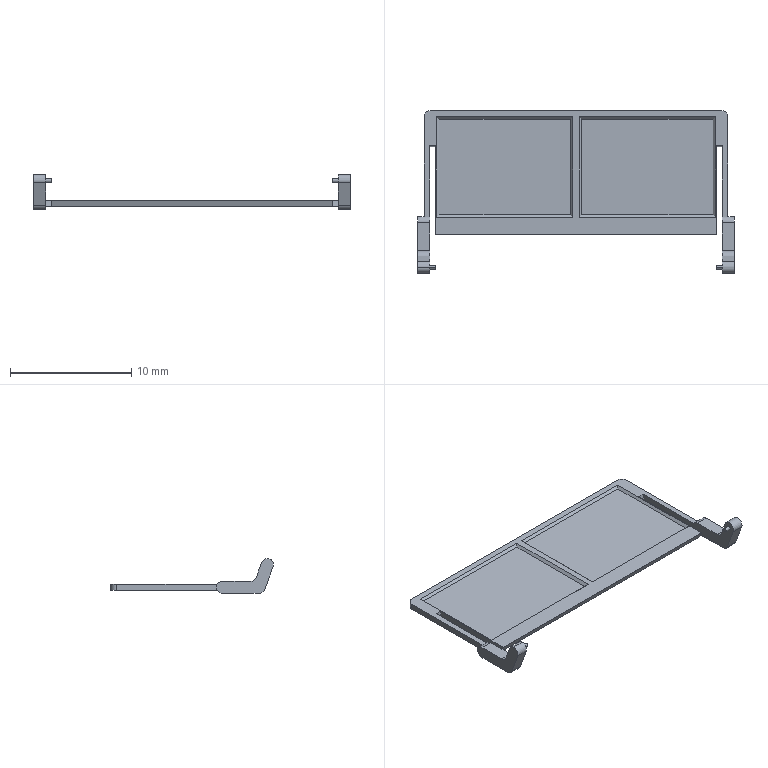Part | SolidWorks | features ICE 4, CutThin 2, Chamfer 1, Extrusion 1, Fillet 1, MirrorPattern 1 | 1 solid | 50 faces | box 26.09 x 13.404 x 2.879 mm | volume 97.812 mm3 | plane 33 | cylinder 17 | commonest cylinder face diameters 1 x11 0.3 x4 20.3 x2
STEP:
#1=CARTESIAN_POINT('',(12.045,-7.814,2.029));
#2=VERTEX_POINT('',#1);
#3=CARTESIAN_POINT('',(12.045,-7.814,1.729));
#4=VERTEX_POINT('',#3);
#5=CARTESIAN_POINT('',(12.045,-7.814,1.879));
#6=DIRECTION('',(-1.,0.,0.));
#7=DIRECTION('',(0.,0.,1.));
#8=AXIS2_PLACEMENT_3D('',#5,#6,#7);
#9=CIRCLE('',#8,0.15);
#10=EDGE_CURVE('',#2,#4,#9,.T.);
#11=ORIENTED_EDGE('',*,*,#10,.T.);
#12=CARTESIAN_POINT('',(11.545,-7.814,1.729));
#13=VERTEX_POINT('',#12);
#14=CARTESIAN_POINT('',(12.045,-7.814,1.729));
#15=DIRECTION('',(-1.,0.,0.));
#16=VECTOR('',#15,1000.);
#17=LINE('',#14,#16);
#18=EDGE_CURVE('',#4,#13,#17,.T.);
#19=ORIENTED_EDGE('',*,*,#18,.T.);
#20=CARTESIAN_POINT('',(11.545,-7.814,2.029));
#21=VERTEX_POINT('',#20);
#22=CARTESIAN_POINT('',(11.545,-7.814,1.879));
#23=DIRECTION('',(-1.,0.,0.));
#24=DIRECTION('',(0.,0.,1.));
#25=AXIS2_PLACEMENT_3D('',#22,#23,#24);
#26=CIRCLE('',#25,0.15);
#27=EDGE_CURVE('',#21,#13,#26,.T.);
#28=ORIENTED_EDGE('',*,*,#27,.F.);
#29=CARTESIAN_POINT('',(12.045,-7.814,2.029));
#30=DIRECTION('',(-1.,0.,0.));
#31=VECTOR('',#30,1000.);
#32=LINE('',#29,#31);
#33=EDGE_CURVE('',#2,#21,#32,.T.);
#34=ORIENTED_EDGE('',*,*,#33,.F.);
#35=EDGE_LOOP('',(#11,#19,#28,#34));
#36=FACE_OUTER_BOUND('',#35,.T.);
#37=CARTESIAN_POINT('',(12.045,-7.814,1.879));
#38=DIRECTION('',(-1.,0.,0.));
#39=DIRECTION('',(0.,0.,1.));
#40=AXIS2_PLACEMENT_3D('',#37,#38,#39);
#41=CYLINDRICAL_SURFACE('',#40,0.15);
#42=ADVANCED_FACE('',(#36),#41,.T.);
#43=CARTESIAN_POINT('',(-12.045,-7.814,1.729));
#44=VERTEX_POINT('',#43);
#45=CARTESIAN_POINT('',(-12.045,-7.814,2.029));
#46=VERTEX_POINT('',#45);
#47=CARTESIAN_POINT('',(-12.045,-7.814,1.879));
#48=DIRECTION('',(1.,0.,0.));
#49=DIRECTION('',(0.,0.,-1.));
#50=AXIS2_PLACEMENT_3D('',#47,#48,#49);
#51=CIRCLE('',#50,0.15);
#52=EDGE_CURVE('',#44,#46,#51,.T.);
#53=ORIENTED_EDGE('',*,*,#52,.T.);
#54=CARTESIAN_POINT('',(-11.545,-7.814,2.029));
#55=VERTEX_POINT('',#54);
#56=CARTESIAN_POINT('',(-12.045,-7.814,2.029));
#57=DIRECTION('',(1.,0.,0.));
#58=VECTOR('',#57,1000.);
#59=LINE('',#56,#58);
#60=EDGE_CURVE('',#46,#55,#59,.T.);
#61=ORIENTED_EDGE('',*,*,#60,.T.);
#62=CARTESIAN_POINT('',(-11.545,-7.814,1.729));
#63=VERTEX_POINT('',#62);
#64=CARTESIAN_POINT('',(-11.545,-7.814,1.879));
#65=DIRECTION('',(1.,0.,0.));
#66=DIRECTION('',(0.,0.,-1.));
#67=AXIS2_PLACEMENT_3D('',#64,#65,#66);
#68=CIRCLE('',#67,0.15);
#69=EDGE_CURVE('',#63,#55,#68,.T.);
#70=ORIENTED_EDGE('',*,*,#69,.F.);
#71=CARTESIAN_POINT('',(-12.045,-7.814,1.729));
#72=DIRECTION('',(1.,0.,0.));
#73=VECTOR('',#72,1000.);
#74=LINE('',#71,#73);
#75=EDGE_CURVE('',#44,#63,#74,.T.);
#76=ORIENTED_EDGE('',*,*,#75,.F.);
#77=EDGE_LOOP('',(#53,#61,#70,#76));
#78=FACE_OUTER_BOUND('',#77,.T.);
#79=CARTESIAN_POINT('',(-12.045,-7.814,1.879));
#80=DIRECTION('',(1.,0.,0.));
#81=DIRECTION('',(0.,0.,-1.));
#82=AXIS2_PLACEMENT_3D('',#79,#80,#81);
#83=CYLINDRICAL_SURFACE('',#82,0.15);
#84=ADVANCED_FACE('',(#78),#83,.T.);
#85=CARTESIAN_POINT('',(-12.045,-7.814,2.379));
#86=VERTEX_POINT('',#85);
#87=CARTESIAN_POINT('',(-12.045,-8.284,1.708));
#88=VERTEX_POINT('',#87);
#89=CARTESIAN_POINT('',(-12.045,-7.814,1.879));
#90=DIRECTION('',(1.,0.,0.));
#91=DIRECTION('',(0.,0.,-1.));
#92=AXIS2_PLACEMENT_3D('',#89,#90,#91);
#93=CIRCLE('',#92,0.5);
#94=EDGE_CURVE('',#86,#88,#93,.T.);
#95=ORIENTED_EDGE('',*,*,#94,.F.);
#96=CARTESIAN_POINT('',(-13.045,-7.814,2.379));
#97=VERTEX_POINT('',#96);
#98=CARTESIAN_POINT('',(-12.045,-7.814,2.379));
#99=DIRECTION('',(-1.,0.,0.));
#100=VECTOR('',#99,1000.);
#101=LINE('',#98,#100);
#102=EDGE_CURVE('',#86,#97,#101,.T.);
#103=ORIENTED_EDGE('',*,*,#102,.T.);
#104=CARTESIAN_POINT('',(-13.045,-8.284,1.708));
#105=VERTEX_POINT('',#104);
#106=CARTESIAN_POINT('',(-13.045,-7.814,1.879));
#107=DIRECTION('',(1.,0.,0.));
#108=DIRECTION('',(0.,0.,-1.));
#109=AXIS2_PLACEMENT_3D('',#106,#107,#108);
#110=CIRCLE('',#109,0.5);
#111=EDGE_CURVE('',#97,#105,#110,.T.);
#112=ORIENTED_EDGE('',*,*,#111,.T.);
#113=CARTESIAN_POINT('',(-12.045,-8.284,1.708));
#114=DIRECTION('',(-1.,0.,0.));
#115=VECTOR('',#114,1000.);
#116=LINE('',#113,#115);
#117=EDGE_CURVE('',#88,#105,#116,.T.);
#118=ORIENTED_EDGE('',*,*,#117,.F.);
#119=EDGE_LOOP('',(#95,#103,#112,#118));
#120=FACE_OUTER_BOUND('',#119,.T.);
#121=CARTESIAN_POINT('',(-12.045,-7.814,1.879));
#122=DIRECTION('',(-1.,0.,0.));
#123=DIRECTION('',(0.,0.,1.));
#124=AXIS2_PLACEMENT_3D('',#121,#122,#123);
#125=CYLINDRICAL_SURFACE('',#124,0.5);
#126=ADVANCED_FACE('',(#120),#125,.T.);
#127=CARTESIAN_POINT('',(12.045,-3.697,-0.25));
#128=VERTEX_POINT('',#127);
#129=CARTESIAN_POINT('',(12.5,-3.697,-0.25));
#130=VERTEX_POINT('',#129);
#131=CARTESIAN_POINT('',(12.045,-3.697,-0.25));
#132=DIRECTION('',(1.,0.,0.));
#133=VECTOR('',#132,1000.);
#134=LINE('',#131,#133);
#135=EDGE_CURVE('',#128,#130,#134,.T.);
#136=ORIENTED_EDGE('',*,*,#135,.F.);
#137=CARTESIAN_POINT('',(12.045,2.11,-0.25));
#138=VERTEX_POINT('',#137);
#139=CARTESIAN_POINT('',(12.045,0.,-0.25));
#140=DIRECTION('',(0.,1.,0.));
#141=VECTOR('',#140,1000.);
#142=LINE('',#139,#141);
#143=EDGE_CURVE('',#128,#138,#142,.T.);
#144=ORIENTED_EDGE('',*,*,#143,.T.);
#145=CARTESIAN_POINT('',(11.545,2.11,-0.25));
#146=VERTEX_POINT('',#145);
#147=CARTESIAN_POINT('',(12.045,2.11,-0.25));
#148=DIRECTION('',(1.,0.,0.));
#149=VECTOR('',#148,1000.);
#150=LINE('',#147,#149);
#151=EDGE_CURVE('',#146,#138,#150,.T.);
#152=ORIENTED_EDGE('',*,*,#151,.F.);
#153=CARTESIAN_POINT('',(11.545,-4.91,-0.25));
#154=VERTEX_POINT('',#153);
#155=CARTESIAN_POINT('',(11.545,0.,-0.25));
#156=DIRECTION('',(0.,1.,0.));
#157=VECTOR('',#156,1000.);
#158=LINE('',#155,#157);
#159=EDGE_CURVE('',#154,#146,#158,.T.);
#160=ORIENTED_EDGE('',*,*,#159,.F.);
#161=CARTESIAN_POINT('',(-11.545,-4.91,-0.25));
#162=VERTEX_POINT('',#161);
#163=CARTESIAN_POINT('',(-12.045,-4.91,-0.25));
#164=DIRECTION('',(1.,0.,0.));
#165=VECTOR('',#164,1000.);
#166=LINE('',#163,#165);
#167=EDGE_CURVE('',#162,#154,#166,.T.);
#168=ORIENTED_EDGE('',*,*,#167,.F.);
#169=CARTESIAN_POINT('',(-11.545,2.11,-0.25));
#170=VERTEX_POINT('',#169);
#171=CARTESIAN_POINT('',(-11.545,0.,-0.25));
#172=DIRECTION('',(0.,-1.,0.));
#173=VECTOR('',#172,1000.);
#174=LINE('',#171,#173);
#175=EDGE_CURVE('',#170,#162,#174,.T.);
#176=ORIENTED_EDGE('',*,*,#175,.F.);
#177=CARTESIAN_POINT('',(-12.045,2.11,-0.25));
#178=VERTEX_POINT('',#177);
#179=CARTESIAN_POINT('',(-12.045,2.11,-0.25));
#180=DIRECTION('',(1.,0.,0.));
#181=VECTOR('',#180,1000.);
#182=LINE('',#179,#181);
#183=EDGE_CURVE('',#178,#170,#182,.T.);
#184=ORIENTED_EDGE('',*,*,#183,.F.);
#185=CARTESIAN_POINT('',(-12.045,-3.697,-0.25));
#186=VERTEX_POINT('',#185);
#187=CARTESIAN_POINT('',(-12.045,0.,-0.25));
#188=DIRECTION('',(0.,-1.,0.));
#189=VECTOR('',#188,1000.);
#190=LINE('',#187,#189);
#191=EDGE_CURVE('',#178,#186,#190,.T.);
#192=ORIENTED_EDGE('',*,*,#191,.T.);
#193=CARTESIAN_POINT('',(-12.5,-3.697,-0.25));
#194=VERTEX_POINT('',#193);
#195=CARTESIAN_POINT('',(-12.045,-3.697,-0.25));
#196=DIRECTION('',(-1.,0.,0.));
#197=VECTOR('',#196,1000.);
#198=LINE('',#195,#197);
#199=EDGE_CURVE('',#186,#194,#198,.T.);
#200=ORIENTED_EDGE('',*,*,#199,.T.);
#201=CARTESIAN_POINT('',(-12.5,4.59,-0.25));
#202=VERTEX_POINT('',#201);
#203=CARTESIAN_POINT('',(-12.5,-5.09,-0.25));
#204=DIRECTION('',(0.,-1.,0.));
#205=VECTOR('',#204,1000.);
#206=LINE('',#203,#205);
#207=EDGE_CURVE('',#202,#194,#206,.T.);
#208=ORIENTED_EDGE('',*,*,#207,.F.);
#209=CARTESIAN_POINT('',(-12.,5.09,-0.25));
#210=VERTEX_POINT('',#209);
#211=CARTESIAN_POINT('',(-12.,4.59,-0.25));
#212=DIRECTION('',(0.,0.,-1.));
#213=DIRECTION('',(-1.,0.,0.));
#214=AXIS2_PLACEMENT_3D('',#211,#212,#213);
#215=CIRCLE('',#214,0.5);
#216=EDGE_CURVE('',#202,#210,#215,.T.);
#217=ORIENTED_EDGE('',*,*,#216,.T.);
#218=CARTESIAN_POINT('',(12.,5.09,-0.25));
#219=VERTEX_POINT('',#218);
#220=CARTESIAN_POINT('',(-12.5,5.09,-0.25));
#221=DIRECTION('',(-1.,0.,0.));
#222=VECTOR('',#221,1000.);
#223=LINE('',#220,#222);
#224=EDGE_CURVE('',#219,#210,#223,.T.);
#225=ORIENTED_EDGE('',*,*,#224,.F.);
#226=CARTESIAN_POINT('',(12.5,4.59,-0.25));
#227=VERTEX_POINT('',#226);
#228=CARTESIAN_POINT('',(12.,4.59,-0.25));
#229=DIRECTION('',(0.,0.,-1.));
#230=DIRECTION('',(-1.,0.,0.));
#231=AXIS2_PLACEMENT_3D('',#228,#229,#230);
#232=CIRCLE('',#231,0.5);
#233=EDGE_CURVE('',#219,#227,#232,.T.);
#234=ORIENTED_EDGE('',*,*,#233,.T.);
#235=CARTESIAN_POINT('',(12.5,-5.09,-0.25));
#236=DIRECTION('',(0.,1.,0.));
#237=VECTOR('',#236,1000.);
#238=LINE('',#235,#237);
#239=EDGE_CURVE('',#130,#227,#238,.T.);
#240=ORIENTED_EDGE('',*,*,#239,.F.);
#241=EDGE_LOOP('',(#136,#144,#152,#160,#168,#176,#184,#192,#200,#208,#217,#225,#234,#240));
#242=FACE_OUTER_BOUND('',#241,.T.);
#243=CARTESIAN_POINT('',(0.,0.,-0.25));
#244=DIRECTION('',(0.,0.,-1.));
#245=DIRECTION('',(-1.,0.,0.));
#246=AXIS2_PLACEMENT_3D('',#243,#244,#245);
#247=PLANE('',#246);
#248=ADVANCED_FACE('',(#242),#247,.T.);
#249=CARTESIAN_POINT('',(0.25,4.59,0.25));
#250=VERTEX_POINT('',#249);
#251=CARTESIAN_POINT('',(0.25,-3.69,0.25));
#252=VERTEX_POINT('',#251);
#253=CARTESIAN_POINT('',(0.25,4.59,0.25));
#254=DIRECTION('',(0.,-1.,0.));
#255=VECTOR('',#254,1000.);
#256=LINE('',#253,#255);
#257=EDGE_CURVE('',#250,#252,#256,.T.);
#258=ORIENTED_EDGE('',*,*,#257,.F.);
#259=CARTESIAN_POINT('',(11.5,4.59,0.25));
#260=VERTEX_POINT('',#259);
#261=CARTESIAN_POINT('',(11.5,4.59,0.25));
#262=DIRECTION('',(-1.,0.,0.));
#263=VECTOR('',#262,1000.);
#264=LINE('',#261,#263);
#265=EDGE_CURVE('',#260,#250,#264,.T.);
#266=ORIENTED_EDGE('',*,*,#265,.F.);
#267=CARTESIAN_POINT('',(11.5,-3.69,0.25));
#268=VERTEX_POINT('',#267);
#269=CARTESIAN_POINT('',(11.5,4.59,0.25));
#270=DIRECTION('',(0.,1.,0.));
#271=VECTOR('',#270,1000.);
#272=LINE('',#269,#271);
#273=EDGE_CURVE('',#268,#260,#272,.T.);
#274=ORIENTED_EDGE('',*,*,#273,.F.);
#275=CARTESIAN_POINT('',(11.5,-3.69,0.25));
#276=DIRECTION('',(1.,0.,0.));
#277=VECTOR('',#276,1000.);
#278=LINE('',#275,#277);
#279=EDGE_CURVE('',#252,#268,#278,.T.);
#280=ORIENTED_EDGE('',*,*,#279,.F.);
#281=EDGE_LOOP('',(#258,#266,#274,#280));
#282=FACE_BOUND('',#281,.T.);
#283=CARTESIAN_POINT('',(-11.5,-3.69,0.25));
#284=VERTEX_POINT('',#283);
#285=CARTESIAN_POINT('',(-0.25,-3.69,0.25));
#286=VERTEX_POINT('',#285);
#287=CARTESIAN_POINT('',(-11.5,-3.69,0.25));
#288=DIRECTION('',(1.,0.,0.));
#289=VECTOR('',#288,1000.);
#290=LINE('',#287,#289);
#291=EDGE_CURVE('',#284,#286,#290,.T.);
#292=ORIENTED_EDGE('',*,*,#291,.F.);
#293=CARTESIAN_POINT('',(-11.5,4.59,0.25));
#294=VERTEX_POINT('',#293);
#295=CARTESIAN_POINT('',(-11.5,4.59,0.25));
#296=DIRECTION('',(0.,-1.,0.));
#297=VECTOR('',#296,1000.);
#298=LINE('',#295,#297);
#299=EDGE_CURVE('',#294,#284,#298,.T.);
#300=ORIENTED_EDGE('',*,*,#299,.F.);
#301=CARTESIAN_POINT('',(-0.25,4.59,0.25));
#302=VERTEX_POINT('',#301);
#303=CARTESIAN_POINT('',(-11.5,4.59,0.25));
#304=DIRECTION('',(-1.,0.,0.));
#305=VECTOR('',#304,1000.);
#306=LINE('',#303,#305);
#307=EDGE_CURVE('',#302,#294,#306,.T.);
#308=ORIENTED_EDGE('',*,*,#307,.F.);
#309=CARTESIAN_POINT('',(-0.25,4.59,0.25));
#310=DIRECTION('',(0.,1.,0.));
#311=VECTOR('',#310,1000.);
#312=LINE('',#309,#311);
#313=EDGE_CURVE('',#286,#302,#312,.T.);
#314=ORIENTED_EDGE('',*,*,#313,.F.);
#315=EDGE_LOOP('',(#292,#300,#308,#314));
#316=FACE_BOUND('',#315,.T.);
#317=CARTESIAN_POINT('',(12.045,-3.697,0.25));
#318=VERTEX_POINT('',#317);
#319=CARTESIAN_POINT('',(12.045,2.204,0.25));
#320=VERTEX_POINT('',#319);
#321=CARTESIAN_POINT('',(12.045,0.,0.25));
#322=DIRECTION('',(0.,1.,0.));
#323=VECTOR('',#322,1000.);
#324=LINE('',#321,#323);
#325=EDGE_CURVE('',#318,#320,#324,.T.);
#326=ORIENTED_EDGE('',*,*,#325,.F.);
#327=CARTESIAN_POINT('',(12.5,-3.697,0.25));
#328=VERTEX_POINT('',#327);
#329=CARTESIAN_POINT('',(12.045,-3.697,0.25));
#330=DIRECTION('',(1.,0.,0.));
#331=VECTOR('',#330,1000.);
#332=LINE('',#329,#331);
#333=EDGE_CURVE('',#318,#328,#332,.T.);
#334=ORIENTED_EDGE('',*,*,#333,.T.);
#335=CARTESIAN_POINT('',(12.5,4.59,0.25));
#336=VERTEX_POINT('',#335);
#337=CARTESIAN_POINT('',(12.5,-5.09,0.25));
#338=DIRECTION('',(0.,1.,0.));
#339=VECTOR('',#338,1000.);
#340=LINE('',#337,#339);
#341=EDGE_CURVE('',#328,#336,#340,.T.);
#342=ORIENTED_EDGE('',*,*,#341,.T.);
#343=CARTESIAN_POINT('',(12.,5.09,0.25));
#344=VERTEX_POINT('',#343);
#345=CARTESIAN_POINT('',(12.,4.59,0.25));
#346=DIRECTION('',(0.,0.,1.));
#347=DIRECTION('',(-1.,0.,0.));
#348=AXIS2_PLACEMENT_3D('',#345,#346,#347);
#349=CIRCLE('',#348,0.5);
#350=EDGE_CURVE('',#336,#344,#349,.T.);
#351=ORIENTED_EDGE('',*,*,#350,.T.);
#352=CARTESIAN_POINT('',(-12.,5.09,0.25));
#353=VERTEX_POINT('',#352);
#354=CARTESIAN_POINT('',(-12.5,5.09,0.25));
#355=DIRECTION('',(-1.,0.,0.));
#356=VECTOR('',#355,1000.);
#357=LINE('',#354,#356);
#358=EDGE_CURVE('',#344,#353,#357,.T.);
#359=ORIENTED_EDGE('',*,*,#358,.T.);
#360=CARTESIAN_POINT('',(-12.5,4.59,0.25));
#361=VERTEX_POINT('',#360);
#362=CARTESIAN_POINT('',(-12.,4.59,0.25));
#363=DIRECTION('',(0.,0.,1.));
#364=DIRECTION('',(-1.,0.,0.));
#365=AXIS2_PLACEMENT_3D('',#362,#363,#364);
#366=CIRCLE('',#365,0.5);
#367=EDGE_CURVE('',#353,#361,#366,.T.);
#368=ORIENTED_EDGE('',*,*,#367,.T.);
#369=CARTESIAN_POINT('',(-12.5,-3.697,0.25));
#370=VERTEX_POINT('',#369);
#371=CARTESIAN_POINT('',(-12.5,-5.09,0.25));
#372=DIRECTION('',(0.,-1.,0.));
#373=VECTOR('',#372,1000.);
#374=LINE('',#371,#373);
#375=EDGE_CURVE('',#361,#370,#374,.T.);
#376=ORIENTED_EDGE('',*,*,#375,.T.);
#377=CARTESIAN_POINT('',(-12.045,-3.697,0.25));
#378=VERTEX_POINT('',#377);
#379=CARTESIAN_POINT('',(-12.045,-3.697,0.25));
#380=DIRECTION('',(-1.,0.,0.));
#381=VECTOR('',#380,1000.);
#382=LINE('',#379,#381);
#383=EDGE_CURVE('',#378,#370,#382,.T.);
#384=ORIENTED_EDGE('',*,*,#383,.F.);
#385=CARTESIAN_POINT('',(-12.045,2.204,0.25));
#386=VERTEX_POINT('',#385);
#387=CARTESIAN_POINT('',(-12.045,0.,0.25));
#388=DIRECTION('',(0.,-1.,0.));
#389=VECTOR('',#388,1000.);
#390=LINE('',#387,#389);
#391=EDGE_CURVE('',#386,#378,#390,.T.);
#392=ORIENTED_EDGE('',*,*,#391,.F.);
#393=CARTESIAN_POINT('',(-11.545,2.204,0.25));
#394=VERTEX_POINT('',#393);
#395=CARTESIAN_POINT('',(-12.045,2.204,0.25));
#396=DIRECTION('',(1.,0.,0.));
#397=VECTOR('',#396,1000.);
#398=LINE('',#395,#397);
#399=EDGE_CURVE('',#386,#394,#398,.T.);
#400=ORIENTED_EDGE('',*,*,#399,.T.);
#401=CARTESIAN_POINT('',(-11.545,-5.09,0.25));
#402=VERTEX_POINT('',#401);
#403=CARTESIAN_POINT('',(-11.545,0.,0.25));
#404=DIRECTION('',(0.,-1.,0.));
#405=VECTOR('',#404,1000.);
#406=LINE('',#403,#405);
#407=EDGE_CURVE('',#394,#402,#406,.T.);
#408=ORIENTED_EDGE('',*,*,#407,.T.);
#409=CARTESIAN_POINT('',(11.545,-5.09,0.25));
#410=VERTEX_POINT('',#409);
#411=CARTESIAN_POINT('',(-12.5,-5.09,0.25));
#412=DIRECTION('',(1.,0.,0.));
#413=VECTOR('',#412,1000.);
#414=LINE('',#411,#413);
#415=EDGE_CURVE('',#402,#410,#414,.T.);
#416=ORIENTED_EDGE('',*,*,#415,.T.);
#417=CARTESIAN_POINT('',(11.545,2.204,0.25));
#418=VERTEX_POINT('',#417);
#419=CARTESIAN_POINT('',(11.545,0.,0.25));
#420=DIRECTION('',(0.,1.,0.));
#421=VECTOR('',#420,1000.);
#422=LINE('',#419,#421);
#423=EDGE_CURVE('',#410,#418,#422,.T.);
#424=ORIENTED_EDGE('',*,*,#423,.T.);
#425=CARTESIAN_POINT('',(12.045,2.204,0.25));
#426=DIRECTION('',(1.,0.,0.));
#427=VECTOR('',#426,1000.);
#428=LINE('',#425,#427);
#429=EDGE_CURVE('',#418,#320,#428,.T.);
#430=ORIENTED_EDGE('',*,*,#429,.T.);
#431=EDGE_LOOP('',(#326,#334,#342,#351,#359,#368,#376,#384,#392,#400,#408,#416,#424,#430));
#432=FACE_OUTER_BOUND('',#431,.T.);
#433=CARTESIAN_POINT('',(0.,0.,0.25));
#434=DIRECTION('',(0.,0.,-1.));
#435=DIRECTION('',(-1.,0.,0.));
#436=AXIS2_PLACEMENT_3D('',#433,#434,#435);
#437=PLANE('',#436);
#438=ADVANCED_FACE('',(#282,#316,#432),#437,.F.);
#439=CARTESIAN_POINT('',(11.545,-5.09,0.2445));
#440=VERTEX_POINT('',#439);
#441=CARTESIAN_POINT('',(-11.545,-5.09,0.2445));
#442=VERTEX_POINT('',#441);
#443=CARTESIAN_POINT('',(-12.5,-5.09,0.2445));
#444=DIRECTION('',(-1.,0.,0.));
#445=VECTOR('',#444,1000.);
#446=LINE('',#443,#445);
#447=EDGE_CURVE('',#440,#442,#446,.T.);
#448=ORIENTED_EDGE('',*,*,#447,.F.);
#449=CARTESIAN_POINT('',(11.545,-5.09,0.25));
#450=DIRECTION('',(0.,0.,1.));
#451=VECTOR('',#450,1000.);
#452=LINE('',#449,#451);
#453=EDGE_CURVE('',#440,#410,#452,.T.);
#454=ORIENTED_EDGE('',*,*,#453,.T.);
#455=ORIENTED_EDGE('',*,*,#415,.F.);
#456=CARTESIAN_POINT('',(-11.545,-5.09,0.25));
#457=DIRECTION('',(0.,0.,-1.));
#458=VECTOR('',#457,1000.);
#459=LINE('',#456,#458);
#460=EDGE_CURVE('',#402,#442,#459,.T.);
#461=ORIENTED_EDGE('',*,*,#460,.T.);
#462=EDGE_LOOP('',(#448,#454,#455,#461));
#463=FACE_OUTER_BOUND('',#462,.T.);
#464=CARTESIAN_POINT('',(-12.5,-5.09,0.25));
#465=DIRECTION('',(0.,1.,0.));
#466=DIRECTION('',(-1.,0.,0.));
#467=AXIS2_PLACEMENT_3D('',#464,#465,#466);
#468=PLANE('',#467);
#469=ADVANCED_FACE('',(#463),#468,.F.);
#470=ORIENTED_EDGE('',*,*,#341,.F.);
#471=CARTESIAN_POINT('',(12.5,-4.13,0.));
#472=DIRECTION('',(-1.,0.,0.));
#473=DIRECTION('',(0.,0.,1.));
#474=AXIS2_PLACEMENT_3D('',#471,#472,#473);
#475=CIRCLE('',#474,0.5);
#476=EDGE_CURVE('',#328,#130,#475,.T.);
#477=ORIENTED_EDGE('',*,*,#476,.T.);
#478=ORIENTED_EDGE('',*,*,#239,.T.);
#479=CARTESIAN_POINT('',(12.5,4.59,0.25));
#480=DIRECTION('',(0.,0.,1.));
#481=VECTOR('',#480,1000.);
#482=LINE('',#479,#481);
#483=EDGE_CURVE('',#227,#336,#482,.T.);
#484=ORIENTED_EDGE('',*,*,#483,.T.);
#485=EDGE_LOOP('',(#470,#477,#478,#484));
#486=FACE_OUTER_BOUND('',#485,.T.);
#487=CARTESIAN_POINT('',(12.5,-5.09,0.25));
#488=DIRECTION('',(-1.,0.,0.));
#489=DIRECTION('',(0.,0.,1.));
#490=AXIS2_PLACEMENT_3D('',#487,#488,#489);
#491=PLANE('',#490);
#492=ADVANCED_FACE('',(#486),#491,.F.);
#493=ORIENTED_EDGE('',*,*,#358,.F.);
#494=CARTESIAN_POINT('',(12.,5.09,0.25));
#495=DIRECTION('',(0.,0.,-1.));
#496=VECTOR('',#495,1000.);
#497=LINE('',#494,#496);
#498=EDGE_CURVE('',#344,#219,#497,.T.);
#499=ORIENTED_EDGE('',*,*,#498,.T.);
#500=ORIENTED_EDGE('',*,*,#224,.T.);
#501=CARTESIAN_POINT('',(-12.,5.09,0.25));
#502=DIRECTION('',(0.,0.,1.));
#503=VECTOR('',#502,1000.);
#504=LINE('',#501,#503);
#505=EDGE_CURVE('',#210,#353,#504,.T.);
#506=ORIENTED_EDGE('',*,*,#505,.T.);
#507=EDGE_LOOP('',(#493,#499,#500,#506));
#508=FACE_OUTER_BOUND('',#507,.T.);
#509=CARTESIAN_POINT('',(-12.5,5.09,0.25));
#510=DIRECTION('',(0.,-1.,0.));
#511=DIRECTION('',(1.,0.,0.));
#512=AXIS2_PLACEMENT_3D('',#509,#510,#511);
#513=PLANE('',#512);
#514=ADVANCED_FACE('',(#508),#513,.F.);
#515=CARTESIAN_POINT('',(-12.5,-4.13,0.));
#516=DIRECTION('',(-1.,0.,0.));
#517=DIRECTION('',(0.,0.,-1.));
#518=AXIS2_PLACEMENT_3D('',#515,#516,#517);
#519=CIRCLE('',#518,0.5);
#520=EDGE_CURVE('',#370,#194,#519,.T.);
#521=ORIENTED_EDGE('',*,*,#520,.F.);
#522=ORIENTED_EDGE('',*,*,#375,.F.);
#523=CARTESIAN_POINT('',(-12.5,4.59,0.25));
#524=DIRECTION('',(0.,0.,-1.));
#525=VECTOR('',#524,1000.);
#526=LINE('',#523,#525);
#527=EDGE_CURVE('',#361,#202,#526,.T.);
#528=ORIENTED_EDGE('',*,*,#527,.T.);
#529=ORIENTED_EDGE('',*,*,#207,.T.);
#530=EDGE_LOOP('',(#521,#522,#528,#529));
#531=FACE_OUTER_BOUND('',#530,.T.);
#532=CARTESIAN_POINT('',(-12.5,-5.09,0.25));
#533=DIRECTION('',(1.,0.,0.));
#534=DIRECTION('',(0.,0.,-1.));
#535=AXIS2_PLACEMENT_3D('',#532,#533,#534);
#536=PLANE('',#535);
#537=ADVANCED_FACE('',(#531),#536,.F.);
#538=CARTESIAN_POINT('',(0.45,-3.49,0.05));
#539=VERTEX_POINT('',#538);
#540=CARTESIAN_POINT('',(11.3,-3.49,0.05));
#541=VERTEX_POINT('',#540);
#542=CARTESIAN_POINT('',(0.,-3.49,0.05));
#543=DIRECTION('',(1.,0.,0.));
#544=VECTOR('',#543,1000.);
#545=LINE('',#542,#544);
#546=EDGE_CURVE('',#539,#541,#545,.T.);
#547=ORIENTED_EDGE('',*,*,#546,.T.);
#548=CARTESIAN_POINT('',(11.3,4.39,0.05));
#549=VERTEX_POINT('',#548);
#550=CARTESIAN_POINT('',(11.3,0.,0.05));
#551=DIRECTION('',(0.,1.,0.));
#552=VECTOR('',#551,1000.);
#553=LINE('',#550,#552);
#554=EDGE_CURVE('',#541,#549,#553,.T.);
#555=ORIENTED_EDGE('',*,*,#554,.T.);
#556=CARTESIAN_POINT('',(0.45,4.39,0.05));
#557=VERTEX_POINT('',#556);
#558=CARTESIAN_POINT('',(0.,4.39,0.05));
#559=DIRECTION('',(-1.,0.,0.));
#560=VECTOR('',#559,1000.);
#561=LINE('',#558,#560);
#562=EDGE_CURVE('',#549,#557,#561,.T.);
#563=ORIENTED_EDGE('',*,*,#562,.T.);
#564=CARTESIAN_POINT('',(0.45,0.,0.05));
#565=DIRECTION('',(0.,-1.,0.));
#566=VECTOR('',#565,1000.);
#567=LINE('',#564,#566);
#568=EDGE_CURVE('',#557,#539,#567,.T.);
#569=ORIENTED_EDGE('',*,*,#568,.T.);
#570=EDGE_LOOP('',(#547,#555,#563,#569));
#571=FACE_OUTER_BOUND('',#570,.T.);
#572=CARTESIAN_POINT('',(0.,0.,0.05));
#573=DIRECTION('',(0.,0.,1.));
#574=DIRECTION('',(1.,0.,0.));
#575=AXIS2_PLACEMENT_3D('',#572,#573,#574);
#576=PLANE('',#575);
#577=ADVANCED_FACE('',(#571),#576,.T.);
#578=CARTESIAN_POINT('',(-0.45,-3.49,0.05));
#579=VERTEX_POINT('',#578);
#580=CARTESIAN_POINT('',(-0.45,4.39,0.05));
#581=VERTEX_POINT('',#580);
#582=CARTESIAN_POINT('',(-0.45,0.,0.05));
#583=DIRECTION('',(0.,1.,0.));
#584=VECTOR('',#583,1000.);
#585=LINE('',#582,#584);
#586=EDGE_CURVE('',#579,#581,#585,.T.);
#587=ORIENTED_EDGE('',*,*,#586,.T.);
#588=CARTESIAN_POINT('',(-11.3,4.39,0.05));
#589=VERTEX_POINT('',#588);
#590=CARTESIAN_POINT('',(0.,4.39,0.05));
#591=DIRECTION('',(-1.,0.,0.));
#592=VECTOR('',#591,1000.);
#593=LINE('',#590,#592);
#594=EDGE_CURVE('',#581,#589,#593,.T.);
#595=ORIENTED_EDGE('',*,*,#594,.T.);
#596=CARTESIAN_POINT('',(-11.3,-3.49,0.05));
#597=VERTEX_POINT('',#596);
#598=CARTESIAN_POINT('',(-11.3,0.,0.05));
#599=DIRECTION('',(0.,-1.,0.));
#600=VECTOR('',#599,1000.);
#601=LINE('',#598,#600);
#602=EDGE_CURVE('',#589,#597,#601,.T.);
#603=ORIENTED_EDGE('',*,*,#602,.T.);
#604=CARTESIAN_POINT('',(0.,-3.49,0.05));
#605=DIRECTION('',(1.,0.,0.));
#606=VECTOR('',#605,1000.);
#607=LINE('',#604,#606);
#608=EDGE_CURVE('',#597,#579,#607,.T.);
#609=ORIENTED_EDGE('',*,*,#608,.T.);
#610=EDGE_LOOP('',(#587,#595,#603,#609));
#611=FACE_OUTER_BOUND('',#610,.T.);
#612=CARTESIAN_POINT('',(0.,0.,0.05));
#613=DIRECTION('',(0.,0.,1.));
#614=DIRECTION('',(1.,0.,0.));
#615=AXIS2_PLACEMENT_3D('',#612,#613,#614);
#616=PLANE('',#615);
#617=ADVANCED_FACE('',(#611),#616,.T.);
#618=CARTESIAN_POINT('',(1.913,2.927,-1.413));
#619=DIRECTION('',(0.5774,-0.5774,-0.5774));
#620=VECTOR('',#619,1000.);
#621=LINE('',#618,#620);
#622=EDGE_CURVE('',#250,#557,#621,.T.);
#623=ORIENTED_EDGE('',*,*,#622,.F.);
#624=ORIENTED_EDGE('',*,*,#257,.T.);
#625=CARTESIAN_POINT('',(0.3,-3.64,0.2));
#626=DIRECTION('',(-0.5774,-0.5774,0.5774));
#627=VECTOR('',#626,1000.);
#628=LINE('',#625,#627);
#629=EDGE_CURVE('',#539,#252,#628,.T.);
#630=ORIENTED_EDGE('',*,*,#629,.F.);
#631=ORIENTED_EDGE('',*,*,#568,.F.);
#632=EDGE_LOOP('',(#623,#624,#630,#631));
#633=FACE_OUTER_BOUND('',#632,.T.);
#634=CARTESIAN_POINT('',(0.45,0.,0.05));
#635=DIRECTION('',(-0.7071,0.,-0.7071));
#636=DIRECTION('',(0.,-1.,0.));
#637=AXIS2_PLACEMENT_3D('',#634,#635,#636);
#638=PLANE('',#637);
#639=ADVANCED_FACE('',(#633),#638,.F.);
#640=ORIENTED_EDGE('',*,*,#629,.T.);
#641=ORIENTED_EDGE('',*,*,#279,.T.);
#642=CARTESIAN_POINT('',(10.137,-2.327,-1.113));
#643=DIRECTION('',(0.5774,-0.5774,0.5774));
#644=VECTOR('',#643,1000.);
#645=LINE('',#642,#644);
#646=EDGE_CURVE('',#541,#268,#645,.T.);
#647=ORIENTED_EDGE('',*,*,#646,.F.);
#648=ORIENTED_EDGE('',*,*,#546,.F.);
#649=EDGE_LOOP('',(#640,#641,#647,#648));
#650=FACE_OUTER_BOUND('',#649,.T.);
#651=CARTESIAN_POINT('',(0.,-3.49,0.05));
#652=DIRECTION('',(0.,-0.7071,-0.7071));
#653=DIRECTION('',(1.,0.,0.));
#654=AXIS2_PLACEMENT_3D('',#651,#652,#653);
#655=PLANE('',#654);
#656=ADVANCED_FACE('',(#650),#655,.F.);
#657=ORIENTED_EDGE('',*,*,#622,.T.);
#658=ORIENTED_EDGE('',*,*,#562,.F.);
#659=CARTESIAN_POINT('',(9.837,2.927,-1.413));
#660=DIRECTION('',(-0.5774,-0.5774,-0.5774));
#661=VECTOR('',#660,1000.);
#662=LINE('',#659,#661);
#663=EDGE_CURVE('',#260,#549,#662,.T.);
#664=ORIENTED_EDGE('',*,*,#663,.F.);
#665=ORIENTED_EDGE('',*,*,#265,.T.);
#666=EDGE_LOOP('',(#657,#658,#664,#665));
#667=FACE_OUTER_BOUND('',#666,.T.);
#668=CARTESIAN_POINT('',(0.,4.39,0.05));
#669=DIRECTION('',(0.,0.7071,-0.7071));
#670=DIRECTION('',(-1.,0.,0.));
#671=AXIS2_PLACEMENT_3D('',#668,#669,#670);
#672=PLANE('',#671);
#673=ADVANCED_FACE('',(#667),#672,.F.);
#674=ORIENTED_EDGE('',*,*,#646,.T.);
#675=ORIENTED_EDGE('',*,*,#273,.T.);
#676=ORIENTED_EDGE('',*,*,#663,.T.);
#677=ORIENTED_EDGE('',*,*,#554,.F.);
#678=EDGE_LOOP('',(#674,#675,#676,#677));
#679=FACE_OUTER_BOUND('',#678,.T.);
#680=CARTESIAN_POINT('',(11.3,0.,0.05));
#681=DIRECTION('',(0.7071,0.,-0.7071));
#682=DIRECTION('',(0.,1.,0.));
#683=AXIS2_PLACEMENT_3D('',#680,#681,#682);
#684=PLANE('',#683);
#685=ADVANCED_FACE('',(#679),#684,.F.);
#686=CARTESIAN_POINT('',(-7.533,0.2767,-3.717));
#687=DIRECTION('',(0.5774,0.5774,-0.5774));
#688=VECTOR('',#687,1000.);
#689=LINE('',#686,#688);
#690=EDGE_CURVE('',#284,#597,#689,.T.);
#691=ORIENTED_EDGE('',*,*,#690,.F.);
#692=ORIENTED_EDGE('',*,*,#291,.T.);
#693=CARTESIAN_POINT('',(-1.613,-2.327,-1.113));
#694=DIRECTION('',(0.5774,-0.5774,0.5774));
#695=VECTOR('',#694,1000.);
#696=LINE('',#693,#695);
#697=EDGE_CURVE('',#579,#286,#696,.T.);
#698=ORIENTED_EDGE('',*,*,#697,.F.);
#699=ORIENTED_EDGE('',*,*,#608,.F.);
#700=EDGE_LOOP('',(#691,#692,#698,#699));
#701=FACE_OUTER_BOUND('',#700,.T.);
#702=CARTESIAN_POINT('',(0.,-3.49,0.05));
#703=DIRECTION('',(0.,-0.7071,-0.7071));
#704=DIRECTION('',(1.,0.,0.));
#705=AXIS2_PLACEMENT_3D('',#702,#703,#704);
#706=PLANE('',#705);
#707=ADVANCED_FACE('',(#701),#706,.F.);
#708=ORIENTED_EDGE('',*,*,#697,.T.);
#709=ORIENTED_EDGE('',*,*,#313,.T.);
#710=CARTESIAN_POINT('',(-0.3,4.54,0.2));
#711=DIRECTION('',(0.5774,0.5774,0.5774));
#712=VECTOR('',#711,1000.);
#713=LINE('',#710,#712);
#714=EDGE_CURVE('',#581,#302,#713,.T.);
#715=ORIENTED_EDGE('',*,*,#714,.F.);
#716=ORIENTED_EDGE('',*,*,#586,.F.);
#717=EDGE_LOOP('',(#708,#709,#715,#716));
#718=FACE_OUTER_BOUND('',#717,.T.);
#719=CARTESIAN_POINT('',(-0.45,0.,0.05));
#720=DIRECTION('',(0.7071,0.,-0.7071));
#721=DIRECTION('',(0.,1.,0.));
#722=AXIS2_PLACEMENT_3D('',#719,#720,#721);
#723=PLANE('',#722);
#724=ADVANCED_FACE('',(#718),#723,.F.);
#725=ORIENTED_EDGE('',*,*,#690,.T.);
#726=ORIENTED_EDGE('',*,*,#602,.F.);
#727=CARTESIAN_POINT('',(-7.533,0.6233,-3.717));
#728=DIRECTION('',(0.5774,-0.5774,-0.5774));
#729=VECTOR('',#728,1000.);
#730=LINE('',#727,#729);
#731=EDGE_CURVE('',#294,#589,#730,.T.);
#732=ORIENTED_EDGE('',*,*,#731,.F.);
#733=ORIENTED_EDGE('',*,*,#299,.T.);
#734=EDGE_LOOP('',(#725,#726,#732,#733));
#735=FACE_OUTER_BOUND('',#734,.T.);
#736=CARTESIAN_POINT('',(-11.3,0.,0.05));
#737=DIRECTION('',(-0.7071,0.,-0.7071));
#738=DIRECTION('',(0.,-1.,0.));
#739=AXIS2_PLACEMENT_3D('',#736,#737,#738);
#740=PLANE('',#739);
#741=ADVANCED_FACE('',(#735),#740,.F.);
#742=ORIENTED_EDGE('',*,*,#714,.T.);
#743=ORIENTED_EDGE('',*,*,#307,.T.);
#744=ORIENTED_EDGE('',*,*,#731,.T.);
#745=ORIENTED_EDGE('',*,*,#594,.F.);
#746=EDGE_LOOP('',(#742,#743,#744,#745));
#747=FACE_OUTER_BOUND('',#746,.T.);
#748=CARTESIAN_POINT('',(0.,4.39,0.05));
#749=DIRECTION('',(0.,0.7071,-0.7071));
#750=DIRECTION('',(-1.,0.,0.));
#751=AXIS2_PLACEMENT_3D('',#748,#749,#750);
#752=PLANE('',#751);
#753=ADVANCED_FACE('',(#747),#752,.F.);
#754=ORIENTED_EDGE('',*,*,#350,.F.);
#755=ORIENTED_EDGE('',*,*,#483,.F.);
#756=ORIENTED_EDGE('',*,*,#233,.F.);
#757=ORIENTED_EDGE('',*,*,#498,.F.);
#758=EDGE_LOOP('',(#754,#755,#756,#757));
#759=FACE_OUTER_BOUND('',#758,.T.);
#760=CARTESIAN_POINT('',(12.,4.59,0.25));
#761=DIRECTION('',(0.,0.,-1.));
#762=DIRECTION('',(-1.,0.,0.));
#763=AXIS2_PLACEMENT_3D('',#760,#761,#762);
#764=CYLINDRICAL_SURFACE('',#763,0.5);
#765=ADVANCED_FACE('',(#759),#764,.T.);
#766=ORIENTED_EDGE('',*,*,#367,.F.);
#767=ORIENTED_EDGE('',*,*,#505,.F.);
#768=ORIENTED_EDGE('',*,*,#216,.F.);
#769=ORIENTED_EDGE('',*,*,#527,.F.);
#770=EDGE_LOOP('',(#766,#767,#768,#769));
#771=FACE_OUTER_BOUND('',#770,.T.);
#772=CARTESIAN_POINT('',(-12.,4.59,0.25));
#773=DIRECTION('',(0.,0.,-1.));
#774=DIRECTION('',(-1.,0.,0.));
#775=AXIS2_PLACEMENT_3D('',#772,#773,#774);
#776=CYLINDRICAL_SURFACE('',#775,0.5);
#777=ADVANCED_FACE('',(#771),#776,.T.);
#778=CARTESIAN_POINT('',(-12.045,-4.13,0.5));
#779=VERTEX_POINT('',#778);
#780=CARTESIAN_POINT('',(-12.045,-4.13,0.));
#781=DIRECTION('',(1.,0.,0.));
#782=DIRECTION('',(0.,0.,-1.));
#783=AXIS2_PLACEMENT_3D('',#780,#781,#782);
#784=CIRCLE('',#783,0.5);
#785=EDGE_CURVE('',#378,#779,#784,.T.);
#786=ORIENTED_EDGE('',*,*,#785,.F.);
#787=ORIENTED_EDGE('',*,*,#383,.T.);
#788=ORIENTED_EDGE('',*,*,#520,.T.);
#789=ORIENTED_EDGE('',*,*,#199,.F.);
#790=CARTESIAN_POINT('',(-12.045,-4.13,-0.5));
#791=VERTEX_POINT('',#790);
#792=CARTESIAN_POINT('',(-12.045,-4.13,0.));
#793=DIRECTION('',(1.,0.,0.));
#794=DIRECTION('',(0.,0.,-1.));
#795=AXIS2_PLACEMENT_3D('',#792,#793,#794);
#796=CIRCLE('',#795,0.5);
#797=EDGE_CURVE('',#791,#186,#796,.T.);
#798=ORIENTED_EDGE('',*,*,#797,.F.);
#799=CARTESIAN_POINT('',(-13.045,-4.13,-0.5));
#800=VERTEX_POINT('',#799);
#801=CARTESIAN_POINT('',(-12.045,-4.13,-0.5));
#802=DIRECTION('',(-1.,0.,0.));
#803=VECTOR('',#802,1000.);
#804=LINE('',#801,#803);
#805=EDGE_CURVE('',#791,#800,#804,.T.);
#806=ORIENTED_EDGE('',*,*,#805,.T.);
#807=CARTESIAN_POINT('',(-13.045,-4.13,0.5));
#808=VERTEX_POINT('',#807);
#809=CARTESIAN_POINT('',(-13.045,-4.13,0.));
#810=DIRECTION('',(1.,0.,0.));
#811=DIRECTION('',(0.,0.,-1.));
#812=AXIS2_PLACEMENT_3D('',#809,#810,#811);
#813=CIRCLE('',#812,0.5);
#814=EDGE_CURVE('',#800,#808,#813,.T.);
#815=ORIENTED_EDGE('',*,*,#814,.T.);
#816=CARTESIAN_POINT('',(-12.045,-4.13,0.5));
#817=DIRECTION('',(-1.,0.,0.));
#818=VECTOR('',#817,1000.);
#819=LINE('',#816,#818);
#820=EDGE_CURVE('',#779,#808,#819,.T.);
#821=ORIENTED_EDGE('',*,*,#820,.F.);
#822=EDGE_LOOP('',(#786,#787,#788,#789,#798,#806,#815,#821));
#823=FACE_OUTER_BOUND('',#822,.T.);
#824=CARTESIAN_POINT('',(-12.045,-4.13,0.));
#825=DIRECTION('',(-1.,0.,0.));
#826=DIRECTION('',(0.,0.,1.));
#827=AXIS2_PLACEMENT_3D('',#824,#825,#826);
#828=CYLINDRICAL_SURFACE('',#827,0.5);
#829=ADVANCED_FACE('',(#823),#828,.T.);
#830=ORIENTED_EDGE('',*,*,#797,.T.);
#831=ORIENTED_EDGE('',*,*,#191,.F.);
#832=CARTESIAN_POINT('',(-12.045,-7.814,1.879));
#833=DIRECTION('',(1.,0.,0.));
#834=DIRECTION('',(0.,0.,-1.));
#835=AXIS2_PLACEMENT_3D('',#832,#833,#834);
#836=CIRCLE('',#835,10.15);
#837=EDGE_CURVE('',#178,#386,#836,.T.);
#838=ORIENTED_EDGE('',*,*,#837,.T.);
#839=ORIENTED_EDGE('',*,*,#391,.T.);
#840=ORIENTED_EDGE('',*,*,#785,.T.);
#841=CARTESIAN_POINT('',(-12.045,-6.43,0.5));
#842=VERTEX_POINT('',#841);
#843=CARTESIAN_POINT('',(-12.045,-4.13,0.5));
#844=DIRECTION('',(0.,-1.,0.));
#845=VECTOR('',#844,1000.);
#846=LINE('',#843,#845);
#847=EDGE_CURVE('',#779,#842,#846,.T.);
#848=ORIENTED_EDGE('',*,*,#847,.T.);
#849=CARTESIAN_POINT('',(-12.045,-6.9,0.829));
#850=VERTEX_POINT('',#849);
#851=CARTESIAN_POINT('',(-12.045,-6.43,1.));
#852=DIRECTION('',(-1.,0.,0.));
#853=DIRECTION('',(0.,0.,1.));
#854=AXIS2_PLACEMENT_3D('',#851,#852,#853);
#855=CIRCLE('',#854,0.5);
#856=EDGE_CURVE('',#842,#850,#855,.T.);
#857=ORIENTED_EDGE('',*,*,#856,.T.);
#858=CARTESIAN_POINT('',(-12.045,-7.344,2.05));
#859=VERTEX_POINT('',#858);
#860=CARTESIAN_POINT('',(-12.045,-6.9,0.829));
#861=DIRECTION('',(0.,-0.342,0.9397));
#862=VECTOR('',#861,1000.);
#863=LINE('',#860,#862);
#864=EDGE_CURVE('',#850,#859,#863,.T.);
#865=ORIENTED_EDGE('',*,*,#864,.T.);
#866=CARTESIAN_POINT('',(-12.045,-7.814,1.879));
#867=DIRECTION('',(1.,0.,0.));
#868=DIRECTION('',(0.,0.,-1.));
#869=AXIS2_PLACEMENT_3D('',#866,#867,#868);
#870=CIRCLE('',#869,0.5);
#871=EDGE_CURVE('',#859,#86,#870,.T.);
#872=ORIENTED_EDGE('',*,*,#871,.T.);
#873=ORIENTED_EDGE('',*,*,#94,.T.);
#874=CARTESIAN_POINT('',(-12.045,-7.6,-0.171));
#875=VERTEX_POINT('',#874);
#876=CARTESIAN_POINT('',(-12.045,-7.6,-0.171));
#877=DIRECTION('',(0.,0.342,-0.9397));
#878=VECTOR('',#877,1000.);
#879=LINE('',#876,#878);
#880=EDGE_CURVE('',#88,#875,#879,.T.);
#881=ORIENTED_EDGE('',*,*,#880,.T.);
#882=CARTESIAN_POINT('',(-12.045,-7.13,-0.5));
#883=VERTEX_POINT('',#882);
#884=CARTESIAN_POINT('',(-12.045,-7.13,0.));
#885=DIRECTION('',(1.,0.,0.));
#886=DIRECTION('',(0.,0.,-1.));
#887=AXIS2_PLACEMENT_3D('',#884,#885,#886);
#888=CIRCLE('',#887,0.5);
#889=EDGE_CURVE('',#875,#883,#888,.T.);
#890=ORIENTED_EDGE('',*,*,#889,.T.);
#891=CARTESIAN_POINT('',(-12.045,-4.13,-0.5));
#892=DIRECTION('',(0.,1.,0.));
#893=VECTOR('',#892,1000.);
#894=LINE('',#891,#893);
#895=EDGE_CURVE('',#883,#791,#894,.T.);
#896=ORIENTED_EDGE('',*,*,#895,.T.);
#897=EDGE_LOOP('',(#830,#831,#838,#839,#840,#848,#857,#865,#872,#873,#881,#890,#896));
#898=FACE_OUTER_BOUND('',#897,.T.);
#899=ORIENTED_EDGE('',*,*,#52,.F.);
#900=CARTESIAN_POINT('',(-12.045,-7.814,1.879));
#901=DIRECTION('',(1.,0.,0.));
#902=DIRECTION('',(0.,0.,-1.));
#903=AXIS2_PLACEMENT_3D('',#900,#901,#902);
#904=CIRCLE('',#903,0.15);
#905=EDGE_CURVE('',#46,#44,#904,.T.);
#906=ORIENTED_EDGE('',*,*,#905,.F.);
#907=EDGE_LOOP('',(#899,#906));
#908=FACE_BOUND('',#907,.T.);
#909=CARTESIAN_POINT('',(-12.045,-6.43,1.));
#910=DIRECTION('',(-1.,0.,0.));
#911=DIRECTION('',(0.,0.,1.));
#912=AXIS2_PLACEMENT_3D('',#909,#910,#911);
#913=PLANE('',#912);
#914=ADVANCED_FACE('',(#898,#908),#913,.F.);
#915=CARTESIAN_POINT('',(-13.045,-6.43,0.5));
#916=VERTEX_POINT('',#915);
#917=CARTESIAN_POINT('',(-13.045,-6.9,0.829));
#918=VERTEX_POINT('',#917);
#919=CARTESIAN_POINT('',(-13.045,-6.43,1.));
#920=DIRECTION('',(-1.,0.,0.));
#921=DIRECTION('',(0.,0.,1.));
#922=AXIS2_PLACEMENT_3D('',#919,#920,#921);
#923=CIRCLE('',#922,0.5);
#924=EDGE_CURVE('',#916,#918,#923,.T.);
#925=ORIENTED_EDGE('',*,*,#924,.T.);
#926=CARTESIAN_POINT('',(-12.045,-6.9,0.829));
#927=DIRECTION('',(-1.,0.,0.));
#928=VECTOR('',#927,1000.);
#929=LINE('',#926,#928);
#930=EDGE_CURVE('',#850,#918,#929,.T.);
#931=ORIENTED_EDGE('',*,*,#930,.F.);
#932=ORIENTED_EDGE('',*,*,#856,.F.);
#933=CARTESIAN_POINT('',(-12.045,-6.43,0.5));
#934=DIRECTION('',(-1.,0.,0.));
#935=VECTOR('',#934,1000.);
#936=LINE('',#933,#935);
#937=EDGE_CURVE('',#842,#916,#936,.T.);
#938=ORIENTED_EDGE('',*,*,#937,.T.);
#939=EDGE_LOOP('',(#925,#931,#932,#938));
#940=FACE_OUTER_BOUND('',#939,.T.);
#941=CARTESIAN_POINT('',(-12.045,-6.43,1.));
#942=DIRECTION('',(-1.,0.,0.));
#943=DIRECTION('',(0.,0.,1.));
#944=AXIS2_PLACEMENT_3D('',#941,#942,#943);
#945=CYLINDRICAL_SURFACE('',#944,0.5);
#946=ADVANCED_FACE('',(#940),#945,.F.);
#947=CARTESIAN_POINT('',(-13.045,-7.344,2.05));
#948=VERTEX_POINT('',#947);
#949=CARTESIAN_POINT('',(-13.045,-6.9,0.829));
#950=DIRECTION('',(0.,-0.342,0.9397));
#951=VECTOR('',#950,1000.);
#952=LINE('',#949,#951);
#953=EDGE_CURVE('',#918,#948,#952,.T.);
#954=ORIENTED_EDGE('',*,*,#953,.T.);
#955=CARTESIAN_POINT('',(-12.045,-7.344,2.05));
#956=DIRECTION('',(-1.,0.,0.));
#957=VECTOR('',#956,1000.);
#958=LINE('',#955,#957);
#959=EDGE_CURVE('',#859,#948,#958,.T.);
#960=ORIENTED_EDGE('',*,*,#959,.F.);
#961=ORIENTED_EDGE('',*,*,#864,.F.);
#962=ORIENTED_EDGE('',*,*,#930,.T.);
#963=EDGE_LOOP('',(#954,#960,#961,#962));
#964=FACE_OUTER_BOUND('',#963,.T.);
#965=CARTESIAN_POINT('',(-12.045,-6.9,0.829));
#966=DIRECTION('',(0.,-0.9397,-0.342));
#967=DIRECTION('',(0.,0.342,-0.9397));
#968=AXIS2_PLACEMENT_3D('',#965,#966,#967);
#969=PLANE('',#968);
#970=ADVANCED_FACE('',(#964),#969,.F.);
#971=ORIENTED_EDGE('',*,*,#102,.F.);
#972=ORIENTED_EDGE('',*,*,#871,.F.);
#973=ORIENTED_EDGE('',*,*,#959,.T.);
#974=CARTESIAN_POINT('',(-13.045,-7.814,1.879));
#975=DIRECTION('',(1.,0.,0.));
#976=DIRECTION('',(0.,0.,-1.));
#977=AXIS2_PLACEMENT_3D('',#974,#975,#976);
#978=CIRCLE('',#977,0.5);
#979=EDGE_CURVE('',#948,#97,#978,.T.);
#980=ORIENTED_EDGE('',*,*,#979,.T.);
#981=EDGE_LOOP('',(#971,#972,#973,#980));
#982=FACE_OUTER_BOUND('',#981,.T.);
#983=CARTESIAN_POINT('',(-12.045,-7.814,1.879));
#984=DIRECTION('',(-1.,0.,0.));
#985=DIRECTION('',(0.,0.,1.));
#986=AXIS2_PLACEMENT_3D('',#983,#984,#985);
#987=CYLINDRICAL_SURFACE('',#986,0.5);
#988=ADVANCED_FACE('',(#982),#987,.T.);
#989=CARTESIAN_POINT('',(-13.045,-7.6,-0.171));
#990=VERTEX_POINT('',#989);
#991=CARTESIAN_POINT('',(-13.045,-7.6,-0.171));
#992=DIRECTION('',(0.,0.342,-0.9397));
#993=VECTOR('',#992,1000.);
#994=LINE('',#991,#993);
#995=EDGE_CURVE('',#105,#990,#994,.T.);
#996=ORIENTED_EDGE('',*,*,#995,.T.);
#997=CARTESIAN_POINT('',(-12.045,-7.6,-0.171));
#998=DIRECTION('',(-1.,0.,0.));
#999=VECTOR('',#998,1000.);
#1000=LINE('',#997,#999);
#1001=EDGE_CURVE('',#875,#990,#1000,.T.);
#1002=ORIENTED_EDGE('',*,*,#1001,.F.);
#1003=ORIENTED_EDGE('',*,*,#880,.F.);
#1004=ORIENTED_EDGE('',*,*,#117,.T.);
#1005=EDGE_LOOP('',(#996,#1002,#1003,#1004));
#1006=FACE_OUTER_BOUND('',#1005,.T.);
#1007=CARTESIAN_POINT('',(-12.045,-7.6,-0.171));
#1008=DIRECTION('',(0.,0.9397,0.342));
#1009=DIRECTION('',(0.,-0.342,0.9397));
#1010=AXIS2_PLACEMENT_3D('',#1007,#1008,#1009);
#1011=PLANE('',#1010);
#1012=ADVANCED_FACE('',(#1006),#1011,.F.);
#1013=CARTESIAN_POINT('',(-13.045,-7.13,-0.5));
#1014=VERTEX_POINT('',#1013);
#1015=CARTESIAN_POINT('',(-13.045,-7.13,0.));
#1016=DIRECTION('',(1.,0.,0.));
#1017=DIRECTION('',(0.,0.,-1.));
#1018=AXIS2_PLACEMENT_3D('',#1015,#1016,#1017);
#1019=CIRCLE('',#1018,0.5);
#1020=EDGE_CURVE('',#990,#1014,#1019,.T.);
#1021=ORIENTED_EDGE('',*,*,#1020,.T.);
#1022=CARTESIAN_POINT('',(-12.045,-7.13,-0.5));
#1023=DIRECTION('',(-1.,0.,0.));
#1024=VECTOR('',#1023,1000.);
#1025=LINE('',#1022,#1024);
#1026=EDGE_CURVE('',#883,#1014,#1025,.T.);
#1027=ORIENTED_EDGE('',*,*,#1026,.F.);
#1028=ORIENTED_EDGE('',*,*,#889,.F.);
#1029=ORIENTED_EDGE('',*,*,#1001,.T.);
#1030=EDGE_LOOP('',(#1021,#1027,#1028,#1029));
#1031=FACE_OUTER_BOUND('',#1030,.T.);
#1032=CARTESIAN_POINT('',(-12.045,-7.13,0.));
#1033=DIRECTION('',(-1.,0.,0.));
#1034=DIRECTION('',(0.,0.,1.));
#1035=AXIS2_PLACEMENT_3D('',#1032,#1033,#1034);
#1036=CYLINDRICAL_SURFACE('',#1035,0.5);
#1037=ADVANCED_FACE('',(#1031),#1036,.T.);
#1038=CARTESIAN_POINT('',(-13.045,-4.13,-0.5));
#1039=DIRECTION('',(0.,1.,0.));
#1040=VECTOR('',#1039,1000.);
#1041=LINE('',#1038,#1040);
#1042=EDGE_CURVE('',#1014,#800,#1041,.T.);
#1043=ORIENTED_EDGE('',*,*,#1042,.T.);
#1044=ORIENTED_EDGE('',*,*,#805,.F.);
#1045=ORIENTED_EDGE('',*,*,#895,.F.);
#1046=ORIENTED_EDGE('',*,*,#1026,.T.);
#1047=EDGE_LOOP('',(#1043,#1044,#1045,#1046));
#1048=FACE_OUTER_BOUND('',#1047,.T.);
#1049=CARTESIAN_POINT('',(-12.045,-4.13,-0.5));
#1050=DIRECTION('',(0.,0.,1.));
#1051=DIRECTION('',(0.,-1.,0.));
#1052=AXIS2_PLACEMENT_3D('',#1049,#1050,#1051);
#1053=PLANE('',#1052);
#1054=ADVANCED_FACE('',(#1048),#1053,.F.);
#1055=CARTESIAN_POINT('',(-13.045,-4.13,0.5));
#1056=DIRECTION('',(0.,-1.,0.));
#1057=VECTOR('',#1056,1000.);
#1058=LINE('',#1055,#1057);
#1059=EDGE_CURVE('',#808,#916,#1058,.T.);
#1060=ORIENTED_EDGE('',*,*,#1059,.T.);
#1061=ORIENTED_EDGE('',*,*,#937,.F.);
#1062=ORIENTED_EDGE('',*,*,#847,.F.);
#1063=ORIENTED_EDGE('',*,*,#820,.T.);
#1064=EDGE_LOOP('',(#1060,#1061,#1062,#1063));
#1065=FACE_OUTER_BOUND('',#1064,.T.);
#1066=CARTESIAN_POINT('',(-12.045,-4.13,0.5));
#1067=DIRECTION('',(0.,0.,-1.));
#1068=DIRECTION('',(0.,1.,0.));
#1069=AXIS2_PLACEMENT_3D('',#1066,#1067,#1068);
#1070=PLANE('',#1069);
#1071=ADVANCED_FACE('',(#1065),#1070,.F.);
#1072=ORIENTED_EDGE('',*,*,#924,.F.);
#1073=ORIENTED_EDGE('',*,*,#1059,.F.);
#1074=ORIENTED_EDGE('',*,*,#814,.F.);
#1075=ORIENTED_EDGE('',*,*,#1042,.F.);
#1076=ORIENTED_EDGE('',*,*,#1020,.F.);
#1077=ORIENTED_EDGE('',*,*,#995,.F.);
#1078=ORIENTED_EDGE('',*,*,#111,.F.);
#1079=ORIENTED_EDGE('',*,*,#979,.F.);
#1080=ORIENTED_EDGE('',*,*,#953,.F.);
#1081=EDGE_LOOP('',(#1072,#1073,#1074,#1075,#1076,#1077,#1078,#1079,#1080));
#1082=FACE_OUTER_BOUND('',#1081,.T.);
#1083=CARTESIAN_POINT('',(-13.045,-6.43,1.));
#1084=DIRECTION('',(-1.,0.,0.));
#1085=DIRECTION('',(0.,0.,1.));
#1086=AXIS2_PLACEMENT_3D('',#1083,#1084,#1085);
#1087=PLANE('',#1086);
#1088=ADVANCED_FACE('',(#1082),#1087,.T.);
#1089=ORIENTED_EDGE('',*,*,#333,.F.);
#1090=CARTESIAN_POINT('',(12.045,-4.13,0.5));
#1091=VERTEX_POINT('',#1090);
#1092=CARTESIAN_POINT('',(12.045,-4.13,0.));
#1093=DIRECTION('',(1.,0.,0.));
#1094=DIRECTION('',(0.,0.,-1.));
#1095=AXIS2_PLACEMENT_3D('',#1092,#1093,#1094);
#1096=CIRCLE('',#1095,0.5);
#1097=EDGE_CURVE('',#318,#1091,#1096,.T.);
#1098=ORIENTED_EDGE('',*,*,#1097,.T.);
#1099=CARTESIAN_POINT('',(13.045,-4.13,0.5));
#1100=VERTEX_POINT('',#1099);
#1101=CARTESIAN_POINT('',(12.045,-4.13,0.5));
#1102=DIRECTION('',(1.,0.,0.));
#1103=VECTOR('',#1102,1000.);
#1104=LINE('',#1101,#1103);
#1105=EDGE_CURVE('',#1091,#1100,#1104,.T.);
#1106=ORIENTED_EDGE('',*,*,#1105,.T.);
#1107=CARTESIAN_POINT('',(13.045,-4.13,-0.5));
#1108=VERTEX_POINT('',#1107);
#1109=CARTESIAN_POINT('',(13.045,-4.13,0.));
#1110=DIRECTION('',(1.,0.,0.));
#1111=DIRECTION('',(0.,0.,-1.));
#1112=AXIS2_PLACEMENT_3D('',#1109,#1110,#1111);
#1113=CIRCLE('',#1112,0.5);
#1114=EDGE_CURVE('',#1108,#1100,#1113,.T.);
#1115=ORIENTED_EDGE('',*,*,#1114,.F.);
#1116=CARTESIAN_POINT('',(12.045,-4.13,-0.5));
#1117=VERTEX_POINT('',#1116);
#1118=CARTESIAN_POINT('',(12.045,-4.13,-0.5));
#1119=DIRECTION('',(1.,0.,0.));
#1120=VECTOR('',#1119,1000.);
#1121=LINE('',#1118,#1120);
#1122=EDGE_CURVE('',#1117,#1108,#1121,.T.);
#1123=ORIENTED_EDGE('',*,*,#1122,.F.);
#1124=CARTESIAN_POINT('',(12.045,-4.13,0.));
#1125=DIRECTION('',(1.,0.,0.));
#1126=DIRECTION('',(0.,0.,-1.));
#1127=AXIS2_PLACEMENT_3D('',#1124,#1125,#1126);
#1128=CIRCLE('',#1127,0.5);
#1129=EDGE_CURVE('',#1117,#128,#1128,.T.);
#1130=ORIENTED_EDGE('',*,*,#1129,.T.);
#1131=ORIENTED_EDGE('',*,*,#135,.T.);
#1132=ORIENTED_EDGE('',*,*,#476,.F.);
#1133=EDGE_LOOP('',(#1089,#1098,#1106,#1115,#1123,#1130,#1131,#1132));
#1134=FACE_OUTER_BOUND('',#1133,.T.);
#1135=CARTESIAN_POINT('',(12.045,-4.13,0.));
#1136=DIRECTION('',(1.,0.,0.));
#1137=DIRECTION('',(0.,0.,-1.));
#1138=AXIS2_PLACEMENT_3D('',#1135,#1136,#1137);
#1139=CYLINDRICAL_SURFACE('',#1138,0.5);
#1140=ADVANCED_FACE('',(#1134),#1139,.T.);
#1141=ORIENTED_EDGE('',*,*,#1097,.F.);
#1142=ORIENTED_EDGE('',*,*,#325,.T.);
#1143=CARTESIAN_POINT('',(12.045,-7.814,1.879));
#1144=DIRECTION('',(-1.,0.,0.));
#1145=DIRECTION('',(0.,0.,1.));
#1146=AXIS2_PLACEMENT_3D('',#1143,#1144,#1145);
#1147=CIRCLE('',#1146,10.15);
#1148=EDGE_CURVE('',#320,#138,#1147,.T.);
#1149=ORIENTED_EDGE('',*,*,#1148,.T.);
#1150=ORIENTED_EDGE('',*,*,#143,.F.);
#1151=ORIENTED_EDGE('',*,*,#1129,.F.);
#1152=CARTESIAN_POINT('',(12.045,-7.13,-0.5));
#1153=VERTEX_POINT('',#1152);
#1154=CARTESIAN_POINT('',(12.045,-4.13,-0.5));
#1155=DIRECTION('',(0.,1.,0.));
#1156=VECTOR('',#1155,1000.);
#1157=LINE('',#1154,#1156);
#1158=EDGE_CURVE('',#1153,#1117,#1157,.T.);
#1159=ORIENTED_EDGE('',*,*,#1158,.F.);
#1160=CARTESIAN_POINT('',(12.045,-7.6,-0.171));
#1161=VERTEX_POINT('',#1160);
#1162=CARTESIAN_POINT('',(12.045,-7.13,0.));
#1163=DIRECTION('',(1.,0.,0.));
#1164=DIRECTION('',(0.,0.,-1.));
#1165=AXIS2_PLACEMENT_3D('',#1162,#1163,#1164);
#1166=CIRCLE('',#1165,0.5);
#1167=EDGE_CURVE('',#1161,#1153,#1166,.T.);
#1168=ORIENTED_EDGE('',*,*,#1167,.F.);
#1169=CARTESIAN_POINT('',(12.045,-8.284,1.708));
#1170=VERTEX_POINT('',#1169);
#1171=CARTESIAN_POINT('',(12.045,-7.6,-0.171));
#1172=DIRECTION('',(0.,0.342,-0.9397));
#1173=VECTOR('',#1172,1000.);
#1174=LINE('',#1171,#1173);
#1175=EDGE_CURVE('',#1170,#1161,#1174,.T.);
#1176=ORIENTED_EDGE('',*,*,#1175,.F.);
#1177=CARTESIAN_POINT('',(12.045,-7.344,2.05));
#1178=VERTEX_POINT('',#1177);
#1179=CARTESIAN_POINT('',(12.045,-7.814,1.879));
#1180=DIRECTION('',(1.,0.,0.));
#1181=DIRECTION('',(0.,0.,-1.));
#1182=AXIS2_PLACEMENT_3D('',#1179,#1180,#1181);
#1183=CIRCLE('',#1182,0.5);
#1184=EDGE_CURVE('',#1178,#1170,#1183,.T.);
#1185=ORIENTED_EDGE('',*,*,#1184,.F.);
#1186=CARTESIAN_POINT('',(12.045,-6.9,0.829));
#1187=VERTEX_POINT('',#1186);
#1188=CARTESIAN_POINT('',(12.045,-6.9,0.829));
#1189=DIRECTION('',(0.,-0.342,0.9397));
#1190=VECTOR('',#1189,1000.);
#1191=LINE('',#1188,#1190);
#1192=EDGE_CURVE('',#1187,#1178,#1191,.T.);
#1193=ORIENTED_EDGE('',*,*,#1192,.F.);
#1194=CARTESIAN_POINT('',(12.045,-6.43,0.5));
#1195=VERTEX_POINT('',#1194);
#1196=CARTESIAN_POINT('',(12.045,-6.43,1.));
#1197=DIRECTION('',(-1.,0.,0.));
#1198=DIRECTION('',(0.,0.,1.));
#1199=AXIS2_PLACEMENT_3D('',#1196,#1197,#1198);
#1200=CIRCLE('',#1199,0.5);
#1201=EDGE_CURVE('',#1195,#1187,#1200,.T.);
#1202=ORIENTED_EDGE('',*,*,#1201,.F.);
#1203=CARTESIAN_POINT('',(12.045,-4.13,0.5));
#1204=DIRECTION('',(0.,-1.,0.));
#1205=VECTOR('',#1204,1000.);
#1206=LINE('',#1203,#1205);
#1207=EDGE_CURVE('',#1091,#1195,#1206,.T.);
#1208=ORIENTED_EDGE('',*,*,#1207,.F.);
#1209=EDGE_LOOP('',(#1141,#1142,#1149,#1150,#1151,#1159,#1168,#1176,#1185,#1193,#1202,#1208));
#1210=FACE_OUTER_BOUND('',#1209,.T.);
#1211=ORIENTED_EDGE('',*,*,#10,.F.);
#1212=CARTESIAN_POINT('',(12.045,-7.814,1.879));
#1213=DIRECTION('',(-1.,0.,0.));
#1214=DIRECTION('',(0.,0.,1.));
#1215=AXIS2_PLACEMENT_3D('',#1212,#1213,#1214);
#1216=CIRCLE('',#1215,0.15);
#1217=EDGE_CURVE('',#4,#2,#1216,.T.);
#1218=ORIENTED_EDGE('',*,*,#1217,.F.);
#1219=EDGE_LOOP('',(#1211,#1218));
#1220=FACE_BOUND('',#1219,.T.);
#1221=CARTESIAN_POINT('',(12.045,-6.43,1.));
#1222=DIRECTION('',(1.,0.,0.));
#1223=DIRECTION('',(0.,0.,1.));
#1224=AXIS2_PLACEMENT_3D('',#1221,#1222,#1223);
#1225=PLANE('',#1224);
#1226=ADVANCED_FACE('',(#1210,#1220),#1225,.F.);
#1227=CARTESIAN_POINT('',(13.045,-6.43,0.5));
#1228=VERTEX_POINT('',#1227);
#1229=CARTESIAN_POINT('',(13.045,-6.9,0.829));
#1230=VERTEX_POINT('',#1229);
#1231=CARTESIAN_POINT('',(13.045,-6.43,1.));
#1232=DIRECTION('',(-1.,0.,0.));
#1233=DIRECTION('',(0.,0.,1.));
#1234=AXIS2_PLACEMENT_3D('',#1231,#1232,#1233);
#1235=CIRCLE('',#1234,0.5);
#1236=EDGE_CURVE('',#1228,#1230,#1235,.T.);
#1237=ORIENTED_EDGE('',*,*,#1236,.F.);
#1238=CARTESIAN_POINT('',(12.045,-6.43,0.5));
#1239=DIRECTION('',(1.,0.,0.));
#1240=VECTOR('',#1239,1000.);
#1241=LINE('',#1238,#1240);
#1242=EDGE_CURVE('',#1195,#1228,#1241,.T.);
#1243=ORIENTED_EDGE('',*,*,#1242,.F.);
#1244=ORIENTED_EDGE('',*,*,#1201,.T.);
#1245=CARTESIAN_POINT('',(12.045,-6.9,0.829));
#1246=DIRECTION('',(1.,0.,0.));
#1247=VECTOR('',#1246,1000.);
#1248=LINE('',#1245,#1247);
#1249=EDGE_CURVE('',#1187,#1230,#1248,.T.);
#1250=ORIENTED_EDGE('',*,*,#1249,.T.);
#1251=EDGE_LOOP('',(#1237,#1243,#1244,#1250));
#1252=FACE_OUTER_BOUND('',#1251,.T.);
#1253=CARTESIAN_POINT('',(12.045,-6.43,1.));
#1254=DIRECTION('',(1.,0.,0.));
#1255=DIRECTION('',(0.,0.,-1.));
#1256=AXIS2_PLACEMENT_3D('',#1253,#1254,#1255);
#1257=CYLINDRICAL_SURFACE('',#1256,0.5);
#1258=ADVANCED_FACE('',(#1252),#1257,.F.);
#1259=CARTESIAN_POINT('',(13.045,-4.13,0.5));
#1260=DIRECTION('',(0.,-1.,0.));
#1261=VECTOR('',#1260,1000.);
#1262=LINE('',#1259,#1261);
#1263=EDGE_CURVE('',#1100,#1228,#1262,.T.);
#1264=ORIENTED_EDGE('',*,*,#1263,.F.);
#1265=ORIENTED_EDGE('',*,*,#1105,.F.);
#1266=ORIENTED_EDGE('',*,*,#1207,.T.);
#1267=ORIENTED_EDGE('',*,*,#1242,.T.);
#1268=EDGE_LOOP('',(#1264,#1265,#1266,#1267));
#1269=FACE_OUTER_BOUND('',#1268,.T.);
#1270=CARTESIAN_POINT('',(12.045,-4.13,0.5));
#1271=DIRECTION('',(0.,0.,1.));
#1272=DIRECTION('',(0.,-1.,0.));
#1273=AXIS2_PLACEMENT_3D('',#1270,#1271,#1272);
#1274=PLANE('',#1273);
#1275=ADVANCED_FACE('',(#1269),#1274,.T.);
#1276=CARTESIAN_POINT('',(13.045,-7.13,-0.5));
#1277=VERTEX_POINT('',#1276);
#1278=CARTESIAN_POINT('',(13.045,-4.13,-0.5));
#1279=DIRECTION('',(0.,1.,0.));
#1280=VECTOR('',#1279,1000.);
#1281=LINE('',#1278,#1280);
#1282=EDGE_CURVE('',#1277,#1108,#1281,.T.);
#1283=ORIENTED_EDGE('',*,*,#1282,.F.);
#1284=CARTESIAN_POINT('',(12.045,-7.13,-0.5));
#1285=DIRECTION('',(1.,0.,0.));
#1286=VECTOR('',#1285,1000.);
#1287=LINE('',#1284,#1286);
#1288=EDGE_CURVE('',#1153,#1277,#1287,.T.);
#1289=ORIENTED_EDGE('',*,*,#1288,.F.);
#1290=ORIENTED_EDGE('',*,*,#1158,.T.);
#1291=ORIENTED_EDGE('',*,*,#1122,.T.);
#1292=EDGE_LOOP('',(#1283,#1289,#1290,#1291));
#1293=FACE_OUTER_BOUND('',#1292,.T.);
#1294=CARTESIAN_POINT('',(12.045,-4.13,-0.5));
#1295=DIRECTION('',(0.,0.,-1.));
#1296=DIRECTION('',(0.,1.,0.));
#1297=AXIS2_PLACEMENT_3D('',#1294,#1295,#1296);
#1298=PLANE('',#1297);
#1299=ADVANCED_FACE('',(#1293),#1298,.T.);
#1300=CARTESIAN_POINT('',(13.045,-7.6,-0.171));
#1301=VERTEX_POINT('',#1300);
#1302=CARTESIAN_POINT('',(13.045,-7.13,0.));
#1303=DIRECTION('',(1.,0.,0.));
#1304=DIRECTION('',(0.,0.,-1.));
#1305=AXIS2_PLACEMENT_3D('',#1302,#1303,#1304);
#1306=CIRCLE('',#1305,0.5);
#1307=EDGE_CURVE('',#1301,#1277,#1306,.T.);
#1308=ORIENTED_EDGE('',*,*,#1307,.F.);
#1309=CARTESIAN_POINT('',(12.045,-7.6,-0.171));
#1310=DIRECTION('',(1.,0.,0.));
#1311=VECTOR('',#1310,1000.);
#1312=LINE('',#1309,#1311);
#1313=EDGE_CURVE('',#1161,#1301,#1312,.T.);
#1314=ORIENTED_EDGE('',*,*,#1313,.F.);
#1315=ORIENTED_EDGE('',*,*,#1167,.T.);
#1316=ORIENTED_EDGE('',*,*,#1288,.T.);
#1317=EDGE_LOOP('',(#1308,#1314,#1315,#1316));
#1318=FACE_OUTER_BOUND('',#1317,.T.);
#1319=CARTESIAN_POINT('',(12.045,-7.13,0.));
#1320=DIRECTION('',(1.,0.,0.));
#1321=DIRECTION('',(0.,0.,-1.));
#1322=AXIS2_PLACEMENT_3D('',#1319,#1320,#1321);
#1323=CYLINDRICAL_SURFACE('',#1322,0.5);
#1324=ADVANCED_FACE('',(#1318),#1323,.T.);
#1325=CARTESIAN_POINT('',(13.045,-8.284,1.708));
#1326=VERTEX_POINT('',#1325);
#1327=CARTESIAN_POINT('',(13.045,-7.6,-0.171));
#1328=DIRECTION('',(0.,0.342,-0.9397));
#1329=VECTOR('',#1328,1000.);
#1330=LINE('',#1327,#1329);
#1331=EDGE_CURVE('',#1326,#1301,#1330,.T.);
#1332=ORIENTED_EDGE('',*,*,#1331,.F.);
#1333=CARTESIAN_POINT('',(12.045,-8.284,1.708));
#1334=DIRECTION('',(1.,0.,0.));
#1335=VECTOR('',#1334,1000.);
#1336=LINE('',#1333,#1335);
#1337=EDGE_CURVE('',#1170,#1326,#1336,.T.);
#1338=ORIENTED_EDGE('',*,*,#1337,.F.);
#1339=ORIENTED_EDGE('',*,*,#1175,.T.);
#1340=ORIENTED_EDGE('',*,*,#1313,.T.);
#1341=EDGE_LOOP('',(#1332,#1338,#1339,#1340));
#1342=FACE_OUTER_BOUND('',#1341,.T.);
#1343=CARTESIAN_POINT('',(12.045,-7.6,-0.171));
#1344=DIRECTION('',(0.,-0.9397,-0.342));
#1345=DIRECTION('',(0.,0.342,-0.9397));
#1346=AXIS2_PLACEMENT_3D('',#1343,#1344,#1345);
#1347=PLANE('',#1346);
#1348=ADVANCED_FACE('',(#1342),#1347,.T.);
#1349=CARTESIAN_POINT('',(13.045,-7.344,2.05));
#1350=VERTEX_POINT('',#1349);
#1351=CARTESIAN_POINT('',(13.045,-7.814,1.879));
#1352=DIRECTION('',(1.,0.,0.));
#1353=DIRECTION('',(0.,0.,-1.));
#1354=AXIS2_PLACEMENT_3D('',#1351,#1352,#1353);
#1355=CIRCLE('',#1354,0.5);
#1356=EDGE_CURVE('',#1350,#1326,#1355,.T.);
#1357=ORIENTED_EDGE('',*,*,#1356,.F.);
#1358=CARTESIAN_POINT('',(12.045,-7.344,2.05));
#1359=DIRECTION('',(1.,0.,0.));
#1360=VECTOR('',#1359,1000.);
#1361=LINE('',#1358,#1360);
#1362=EDGE_CURVE('',#1178,#1350,#1361,.T.);
#1363=ORIENTED_EDGE('',*,*,#1362,.F.);
#1364=ORIENTED_EDGE('',*,*,#1184,.T.);
#1365=ORIENTED_EDGE('',*,*,#1337,.T.);
#1366=EDGE_LOOP('',(#1357,#1363,#1364,#1365));
#1367=FACE_OUTER_BOUND('',#1366,.T.);
#1368=CARTESIAN_POINT('',(12.045,-7.814,1.879));
#1369=DIRECTION('',(1.,0.,0.));
#1370=DIRECTION('',(0.,0.,-1.));
#1371=AXIS2_PLACEMENT_3D('',#1368,#1369,#1370);
#1372=CYLINDRICAL_SURFACE('',#1371,0.5);
#1373=ADVANCED_FACE('',(#1367),#1372,.T.);
#1374=CARTESIAN_POINT('',(13.045,-6.9,0.829));
#1375=DIRECTION('',(0.,-0.342,0.9397));
#1376=VECTOR('',#1375,1000.);
#1377=LINE('',#1374,#1376);
#1378=EDGE_CURVE('',#1230,#1350,#1377,.T.);
#1379=ORIENTED_EDGE('',*,*,#1378,.F.);
#1380=ORIENTED_EDGE('',*,*,#1249,.F.);
#1381=ORIENTED_EDGE('',*,*,#1192,.T.);
#1382=ORIENTED_EDGE('',*,*,#1362,.T.);
#1383=EDGE_LOOP('',(#1379,#1380,#1381,#1382));
#1384=FACE_OUTER_BOUND('',#1383,.T.);
#1385=CARTESIAN_POINT('',(12.045,-6.9,0.829));
#1386=DIRECTION('',(0.,0.9397,0.342));
#1387=DIRECTION('',(0.,-0.342,0.9397));
#1388=AXIS2_PLACEMENT_3D('',#1385,#1386,#1387);
#1389=PLANE('',#1388);
#1390=ADVANCED_FACE('',(#1384),#1389,.T.);
#1391=ORIENTED_EDGE('',*,*,#1236,.T.);
#1392=ORIENTED_EDGE('',*,*,#1378,.T.);
#1393=ORIENTED_EDGE('',*,*,#1356,.T.);
#1394=ORIENTED_EDGE('',*,*,#1331,.T.);
#1395=ORIENTED_EDGE('',*,*,#1307,.T.);
#1396=ORIENTED_EDGE('',*,*,#1282,.T.);
#1397=ORIENTED_EDGE('',*,*,#1114,.T.);
#1398=ORIENTED_EDGE('',*,*,#1263,.T.);
#1399=EDGE_LOOP('',(#1391,#1392,#1393,#1394,#1395,#1396,#1397,#1398));
#1400=FACE_OUTER_BOUND('',#1399,.T.);
#1401=CARTESIAN_POINT('',(13.045,-6.43,1.));
#1402=DIRECTION('',(1.,0.,0.));
#1403=DIRECTION('',(0.,0.,1.));
#1404=AXIS2_PLACEMENT_3D('',#1401,#1402,#1403);
#1405=PLANE('',#1404);
#1406=ADVANCED_FACE('',(#1400),#1405,.T.);
#1407=CARTESIAN_POINT('',(11.545,-4.91,-0.25));
#1408=DIRECTION('',(0.,0.342,-0.9397));
#1409=VECTOR('',#1408,1000.);
#1410=LINE('',#1407,#1409);
#1411=EDGE_CURVE('',#440,#154,#1410,.T.);
#1412=ORIENTED_EDGE('',*,*,#1411,.F.);
#1413=ORIENTED_EDGE('',*,*,#447,.T.);
#1414=CARTESIAN_POINT('',(-11.545,-4.91,-0.25));
#1415=DIRECTION('',(0.,-0.342,0.9397));
#1416=VECTOR('',#1415,1000.);
#1417=LINE('',#1414,#1416);
#1418=EDGE_CURVE('',#162,#442,#1417,.T.);
#1419=ORIENTED_EDGE('',*,*,#1418,.F.);
#1420=ORIENTED_EDGE('',*,*,#167,.T.);
#1421=EDGE_LOOP('',(#1412,#1413,#1419,#1420));
#1422=FACE_OUTER_BOUND('',#1421,.T.);
#1423=CARTESIAN_POINT('',(-12.045,-4.91,-0.25));
#1424=DIRECTION('',(0.,-0.9397,-0.342));
#1425=DIRECTION('',(0.,0.342,-0.9397));
#1426=AXIS2_PLACEMENT_3D('',#1423,#1424,#1425);
#1427=PLANE('',#1426);
#1428=ADVANCED_FACE('',(#1422),#1427,.T.);
#1429=CARTESIAN_POINT('',(-11.545,-7.814,1.879));
#1430=DIRECTION('',(1.,0.,0.));
#1431=DIRECTION('',(0.,0.,-1.));
#1432=AXIS2_PLACEMENT_3D('',#1429,#1430,#1431);
#1433=CIRCLE('',#1432,10.15);
#1434=EDGE_CURVE('',#170,#394,#1433,.T.);
#1435=ORIENTED_EDGE('',*,*,#1434,.F.);
#1436=ORIENTED_EDGE('',*,*,#175,.T.);
#1437=ORIENTED_EDGE('',*,*,#1418,.T.);
#1438=ORIENTED_EDGE('',*,*,#460,.F.);
#1439=ORIENTED_EDGE('',*,*,#407,.F.);
#1440=EDGE_LOOP('',(#1435,#1436,#1437,#1438,#1439));
#1441=FACE_OUTER_BOUND('',#1440,.T.);
#1442=CARTESIAN_POINT('',(-11.545,-7.814,1.879));
#1443=DIRECTION('',(1.,0.,0.));
#1444=DIRECTION('',(0.,0.,-1.));
#1445=AXIS2_PLACEMENT_3D('',#1442,#1443,#1444);
#1446=PLANE('',#1445);
#1447=ADVANCED_FACE('',(#1441),#1446,.F.);
#1448=ORIENTED_EDGE('',*,*,#183,.T.);
#1449=ORIENTED_EDGE('',*,*,#1434,.T.);
#1450=ORIENTED_EDGE('',*,*,#399,.F.);
#1451=ORIENTED_EDGE('',*,*,#837,.F.);
#1452=EDGE_LOOP('',(#1448,#1449,#1450,#1451));
#1453=FACE_OUTER_BOUND('',#1452,.T.);
#1454=CARTESIAN_POINT('',(-12.045,-7.814,1.879));
#1455=DIRECTION('',(1.,0.,0.));
#1456=DIRECTION('',(0.,0.,-1.));
#1457=AXIS2_PLACEMENT_3D('',#1454,#1455,#1456);
#1458=CYLINDRICAL_SURFACE('',#1457,10.15);
#1459=ADVANCED_FACE('',(#1453),#1458,.F.);
#1460=ORIENTED_EDGE('',*,*,#60,.F.);
#1461=ORIENTED_EDGE('',*,*,#905,.T.);
#1462=ORIENTED_EDGE('',*,*,#75,.T.);
#1463=CARTESIAN_POINT('',(-11.545,-7.814,1.879));
#1464=DIRECTION('',(1.,0.,0.));
#1465=DIRECTION('',(0.,0.,-1.));
#1466=AXIS2_PLACEMENT_3D('',#1463,#1464,#1465);
#1467=CIRCLE('',#1466,0.15);
#1468=EDGE_CURVE('',#55,#63,#1467,.T.);
#1469=ORIENTED_EDGE('',*,*,#1468,.F.);
#1470=EDGE_LOOP('',(#1460,#1461,#1462,#1469));
#1471=FACE_OUTER_BOUND('',#1470,.T.);
#1472=CARTESIAN_POINT('',(-12.045,-7.814,1.879));
#1473=DIRECTION('',(1.,0.,0.));
#1474=DIRECTION('',(0.,0.,-1.));
#1475=AXIS2_PLACEMENT_3D('',#1472,#1473,#1474);
#1476=CYLINDRICAL_SURFACE('',#1475,0.15);
#1477=ADVANCED_FACE('',(#1471),#1476,.T.);
#1478=ORIENTED_EDGE('',*,*,#69,.T.);
#1479=ORIENTED_EDGE('',*,*,#1468,.T.);
#1480=EDGE_LOOP('',(#1478,#1479));
#1481=FACE_OUTER_BOUND('',#1480,.T.);
#1482=CARTESIAN_POINT('',(-11.545,-7.814,1.879));
#1483=DIRECTION('',(1.,0.,0.));
#1484=DIRECTION('',(0.,0.,-1.));
#1485=AXIS2_PLACEMENT_3D('',#1482,#1483,#1484);
#1486=PLANE('',#1485);
#1487=ADVANCED_FACE('',(#1481),#1486,.T.);
#1488=ORIENTED_EDGE('',*,*,#159,.T.);
#1489=CARTESIAN_POINT('',(11.545,-7.814,1.879));
#1490=DIRECTION('',(-1.,0.,0.));
#1491=DIRECTION('',(0.,0.,1.));
#1492=AXIS2_PLACEMENT_3D('',#1489,#1490,#1491);
#1493=CIRCLE('',#1492,10.15);
#1494=EDGE_CURVE('',#418,#146,#1493,.T.);
#1495=ORIENTED_EDGE('',*,*,#1494,.F.);
#1496=ORIENTED_EDGE('',*,*,#423,.F.);
#1497=ORIENTED_EDGE('',*,*,#453,.F.);
#1498=ORIENTED_EDGE('',*,*,#1411,.T.);
#1499=EDGE_LOOP('',(#1488,#1495,#1496,#1497,#1498));
#1500=FACE_OUTER_BOUND('',#1499,.T.);
#1501=CARTESIAN_POINT('',(11.545,-7.814,1.879));
#1502=DIRECTION('',(-1.,0.,0.));
#1503=DIRECTION('',(0.,0.,1.));
#1504=AXIS2_PLACEMENT_3D('',#1501,#1502,#1503);
#1505=PLANE('',#1504);
#1506=ADVANCED_FACE('',(#1500),#1505,.F.);
#1507=ORIENTED_EDGE('',*,*,#151,.T.);
#1508=ORIENTED_EDGE('',*,*,#1148,.F.);
#1509=ORIENTED_EDGE('',*,*,#429,.F.);
#1510=ORIENTED_EDGE('',*,*,#1494,.T.);
#1511=EDGE_LOOP('',(#1507,#1508,#1509,#1510));
#1512=FACE_OUTER_BOUND('',#1511,.T.);
#1513=CARTESIAN_POINT('',(12.045,-7.814,1.879));
#1514=DIRECTION('',(-1.,0.,0.));
#1515=DIRECTION('',(0.,0.,1.));
#1516=AXIS2_PLACEMENT_3D('',#1513,#1514,#1515);
#1517=CYLINDRICAL_SURFACE('',#1516,10.15);
#1518=ADVANCED_FACE('',(#1512),#1517,.F.);
#1519=ORIENTED_EDGE('',*,*,#18,.F.);
#1520=ORIENTED_EDGE('',*,*,#1217,.T.);
#1521=ORIENTED_EDGE('',*,*,#33,.T.);
#1522=CARTESIAN_POINT('',(11.545,-7.814,1.879));
#1523=DIRECTION('',(-1.,0.,0.));
#1524=DIRECTION('',(0.,0.,1.));
#1525=AXIS2_PLACEMENT_3D('',#1522,#1523,#1524);
#1526=CIRCLE('',#1525,0.15);
#1527=EDGE_CURVE('',#13,#21,#1526,.T.);
#1528=ORIENTED_EDGE('',*,*,#1527,.F.);
#1529=EDGE_LOOP('',(#1519,#1520,#1521,#1528));
#1530=FACE_OUTER_BOUND('',#1529,.T.);
#1531=CARTESIAN_POINT('',(12.045,-7.814,1.879));
#1532=DIRECTION('',(-1.,0.,0.));
#1533=DIRECTION('',(0.,0.,1.));
#1534=AXIS2_PLACEMENT_3D('',#1531,#1532,#1533);
#1535=CYLINDRICAL_SURFACE('',#1534,0.15);
#1536=ADVANCED_FACE('',(#1530),#1535,.T.);
#1537=ORIENTED_EDGE('',*,*,#27,.T.);
#1538=ORIENTED_EDGE('',*,*,#1527,.T.);
#1539=EDGE_LOOP('',(#1537,#1538));
#1540=FACE_OUTER_BOUND('',#1539,.T.);
#1541=CARTESIAN_POINT('',(11.545,-7.814,1.879));
#1542=DIRECTION('',(-1.,0.,0.));
#1543=DIRECTION('',(0.,0.,-1.));
#1544=AXIS2_PLACEMENT_3D('',#1541,#1542,#1543);
#1545=PLANE('',#1544);
#1546=ADVANCED_FACE('',(#1540),#1545,.T.);
#1547=CLOSED_SHELL('',(#42,#84,#126,#248,#438,#469,#492,#514,#537,#577,#617,#639,#656,#673,#685,#707,#724,#741,#753,#765,#777,#829,#914,#946,#970,#988,#1012,#1037,#1054,#1071,#1088,#1140,#1226,#1258,#1275,#1299,#1324,#1348,#1373,#1390,#1406,#1428,#1447,#1459,#1477,#1487,#1506,#1518,#1536,#1546));
#1548=MANIFOLD_SOLID_BREP('',#1547);
#1549=CARTESIAN_POINT('',(0.,0.,0.));
#1550=DIRECTION('',(0.,0.,1.));
#1551=DIRECTION('',(1.,0.,0.));
#1552=AXIS2_PLACEMENT_3D('',#1549,#1550,#1551);
#1553=(LENGTH_UNIT()NAMED_UNIT(*)SI_UNIT(.MILLI.,.METRE.));
#1554=UNCERTAINTY_MEASURE_WITH_UNIT(LENGTH_MEASURE(0.00001),#1553,'','');
#1555=(NAMED_UNIT(*)PLANE_ANGLE_UNIT()SI_UNIT($,.RADIAN.));
#1556=(NAMED_UNIT(*)SI_UNIT($,.STERADIAN.)SOLID_ANGLE_UNIT());
#1557=(GEOMETRIC_REPRESENTATION_CONTEXT(3)GLOBAL_UNCERTAINTY_ASSIGNED_CONTEXT((#1554))GLOBAL_UNIT_ASSIGNED_CONTEXT((#1553,#1555,#1556))REPRESENTATION_CONTEXT('',''));
#1558=ADVANCED_BREP_SHAPE_REPRESENTATION('',(#1548,#1552),#1557);